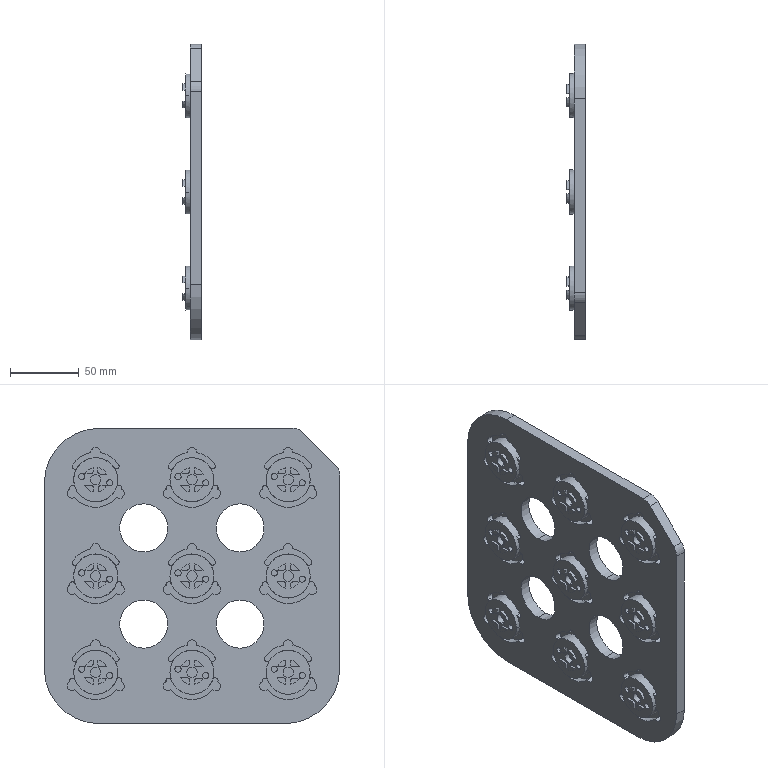Part | SolidWorks | features ICE 7, MoveCopyBody 6, Fillet 3, Cut 2, Chamfer 1, Extrusion 1, LPattern 1, MoveFace 1, Stock 1 | 1 solid | 524 faces | box 13.1 x 214.9 x 214.8 mm | volume 329886 mm3 | cylinder 346 | plane 178 | commonest cylinder face diameters 4 x135 7 x54 4.5 x36 18 x36 40 x36 7.55 x18